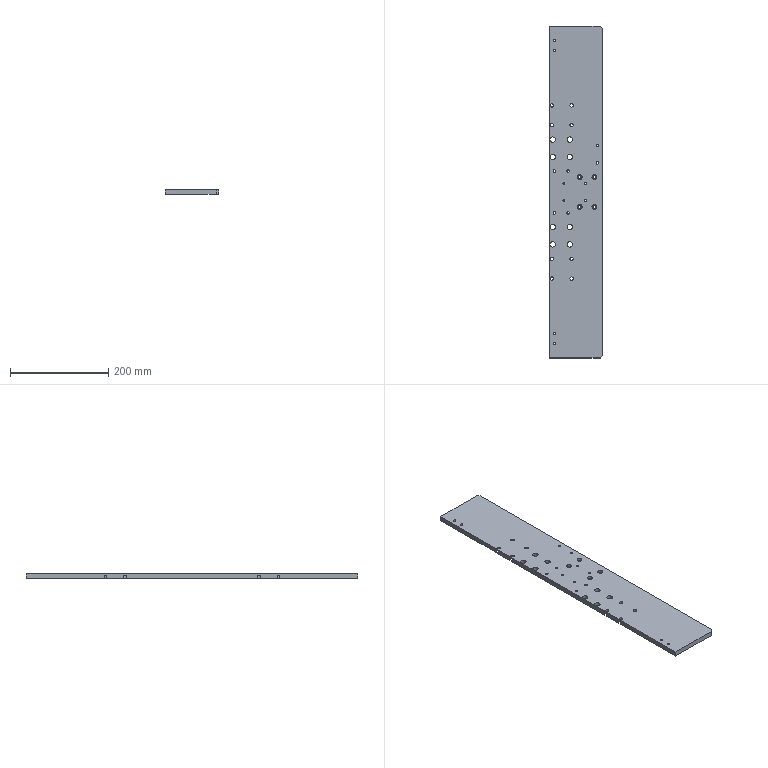Part | SolidWorks | features HoleWzd 6, Chamfer 1, Cut 1, Extrusion 1 | 1 solid | 108 faces | box 108 x 675 x 10 mm | volume 710685 mm3 | cylinder 88 | plane 20 | commonest cylinder face diameters 11 x28 5 x20 6.6 x16 4.2 x8 5.5 x8 10 x8